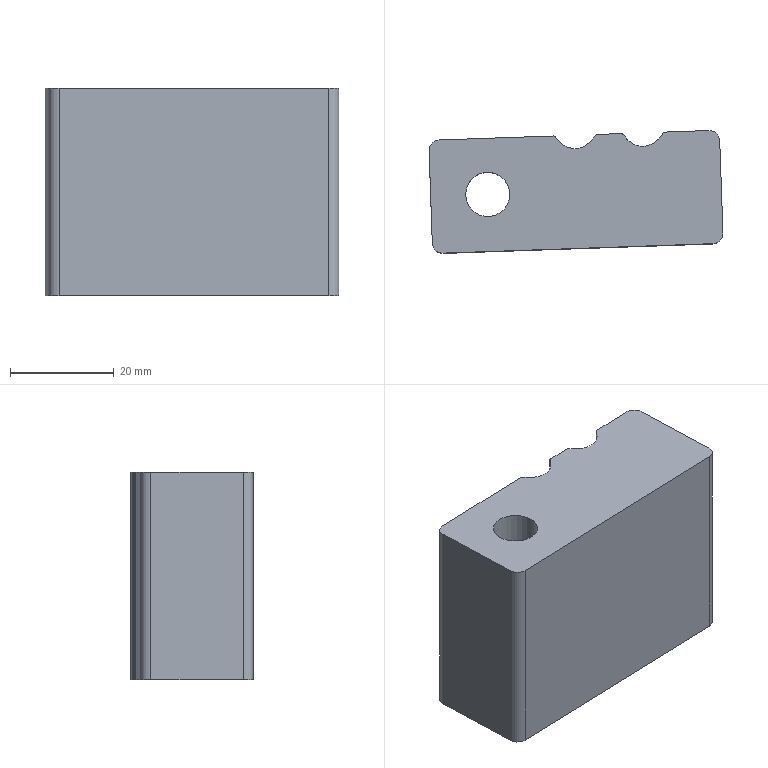Part | NX | features PS-36 2 | 1 solid | 23 faces | box 56.589 x 23.604 x 40 mm | volume 43654 mm3 | cylinder 10 | plane 9 | spline 4 | commonest cylinder face diameters 1 x4 4 x4 8.5 x1 14.5 x1
STEP:
#1=CARTESIAN_POINT('',(3626.085,-818.188,860.716));
#2=VERTEX_POINT('',#1);
#3=CARTESIAN_POINT('',(3648.093,-817.42,860.716));
#4=VERTEX_POINT('',#3);
#5=CARTESIAN_POINT('',(3439.004,-824.721,860.716));
#6=DIRECTION('',(0.9994,0.0349,0.));
#7=VECTOR('',#6,1000.);
#8=LINE('',#5,#7);
#9=EDGE_CURVE('',#2,#4,#8,.T.);
#10=ORIENTED_EDGE('',*,*,#9,.F.);
#11=CARTESIAN_POINT('',(3626.085,-818.188,900.716));
#12=VERTEX_POINT('',#11);
#13=CARTESIAN_POINT('',(3626.085,-818.188,900.716));
#14=DIRECTION('',(0.,0.,1.));
#15=VECTOR('',#14,1000.);
#16=LINE('',#13,#15);
#17=EDGE_CURVE('',#2,#12,#16,.T.);
#18=ORIENTED_EDGE('',*,*,#17,.T.);
#19=CARTESIAN_POINT('',(3648.093,-817.42,900.716));
#20=VERTEX_POINT('',#19);
#21=CARTESIAN_POINT('',(3646.863,-817.463,900.716));
#22=DIRECTION('',(-0.9994,-0.0349,0.));
#23=VECTOR('',#22,1000.);
#24=LINE('',#21,#23);
#25=EDGE_CURVE('',#20,#12,#24,.T.);
#26=ORIENTED_EDGE('',*,*,#25,.F.);
#27=CARTESIAN_POINT('',(3648.093,-817.42,880.716));
#28=DIRECTION('',(0.,0.,1.));
#29=VECTOR('',#28,1000.);
#30=LINE('',#27,#29);
#31=EDGE_CURVE('',#20,#4,#30,.F.);
#32=ORIENTED_EDGE('',*,*,#31,.T.);
#33=EDGE_LOOP('',(#10,#18,#26,#32));
#34=FACE_BOUND('',#33,.T.);
#35=CARTESIAN_POINT('',(3646.863,-817.463,940.716));
#36=DIRECTION('',(0.0349,-0.9994,0.));
#37=DIRECTION('',(-0.9994,-0.0349,0.));
#38=AXIS2_PLACEMENT_3D('',#35,#36,#37);
#39=PLANE('',#38);
#40=ADVANCED_FACE('',(#34),#39,.F.);
#41=CARTESIAN_POINT('',(3648.519,-817.631,900.716));
#42=VERTEX_POINT('',#41);
#43=CARTESIAN_POINT('',(3648.111,-817.92,900.716));
#44=DIRECTION('',(0.,0.,1.));
#45=DIRECTION('',(1.,0.,0.));
#46=AXIS2_PLACEMENT_3D('',#43,#44,#45);
#47=CIRCLE('',#46,0.5);
#48=EDGE_CURVE('',#20,#42,#47,.F.);
#49=ORIENTED_EDGE('',*,*,#48,.T.);
#50=CARTESIAN_POINT('',(3648.519,-817.631,860.716));
#51=VERTEX_POINT('',#50);
#52=CARTESIAN_POINT('',(3648.519,-817.631,860.716));
#53=DIRECTION('',(0.,0.,-1.));
#54=VECTOR('',#53,1000.);
#55=LINE('',#52,#54);
#56=EDGE_CURVE('',#51,#42,#55,.F.);
#57=ORIENTED_EDGE('',*,*,#56,.F.);
#58=CARTESIAN_POINT('',(3648.111,-817.92,860.716));
#59=DIRECTION('',(0.,0.,1.));
#60=DIRECTION('',(1.,0.,0.));
#61=AXIS2_PLACEMENT_3D('',#58,#59,#60);
#62=CIRCLE('',#61,0.5);
#63=EDGE_CURVE('',#4,#51,#62,.F.);
#64=ORIENTED_EDGE('',*,*,#63,.F.);
#65=ORIENTED_EDGE('',*,*,#31,.F.);
#66=EDGE_LOOP('',(#49,#57,#64,#65));
#67=FACE_BOUND('',#66,.T.);
#68=CARTESIAN_POINT('',(3648.111,-817.92,880.716));
#69=DIRECTION('',(0.,0.,-1.));
#70=DIRECTION('',(-1.,0.,0.));
#71=AXIS2_PLACEMENT_3D('',#68,#69,#70);
#72=CYLINDRICAL_SURFACE('',#71,0.5);
#73=ADVANCED_FACE('',(#67),#72,.T.);
#74=CARTESIAN_POINT('',(3652.502,-819.853,900.716));
#75=VERTEX_POINT('',#74);
#76=CARTESIAN_POINT('',(3648.519,-817.631,900.716));
#77=CARTESIAN_POINT('',(3648.979,-818.283,900.716));
#78=CARTESIAN_POINT('',(3650.119,-819.434,900.716));
#79=CARTESIAN_POINT('',(3651.701,-819.895,900.716));
#80=CARTESIAN_POINT('',(3652.502,-819.853,900.716));
#81=B_SPLINE_CURVE_WITH_KNOTS('',3,(#76,#77,#78,#79,#80),.UNSPECIFIED.,.F.,.F.,(4,1,4),(0.,0.002372,0.004744),.UNSPECIFIED.);
#82=EDGE_CURVE('',#42,#75,#81,.T.);
#83=ORIENTED_EDGE('',*,*,#82,.T.);
#84=CARTESIAN_POINT('',(3652.502,-819.853,860.716));
#85=VERTEX_POINT('',#84);
#86=CARTESIAN_POINT('',(3652.502,-819.853,900.716));
#87=CARTESIAN_POINT('',(3652.502,-819.853,887.383));
#88=CARTESIAN_POINT('',(3652.502,-819.853,874.05));
#89=CARTESIAN_POINT('',(3652.502,-819.853,860.716));
#90=B_SPLINE_CURVE_WITH_KNOTS('',3,(#86,#87,#88,#89),.UNSPECIFIED.,.F.,.F.,(4,4),(0.5,1.),.UNSPECIFIED.);
#91=EDGE_CURVE('',#75,#85,#90,.T.);
#92=ORIENTED_EDGE('',*,*,#91,.T.);
#93=CARTESIAN_POINT('',(3652.502,-819.853,860.716));
#94=CARTESIAN_POINT('',(3650.9,-819.937,860.716));
#95=CARTESIAN_POINT('',(3649.439,-818.936,860.716));
#96=CARTESIAN_POINT('',(3648.519,-817.631,860.716));
#97=B_SPLINE_CURVE_WITH_KNOTS('',3,(#93,#94,#95,#96),.UNSPECIFIED.,.F.,.F.,(4,4),(0.,0.004741),.UNSPECIFIED.);
#98=EDGE_CURVE('',#85,#51,#97,.T.);
#99=ORIENTED_EDGE('',*,*,#98,.T.);
#100=ORIENTED_EDGE('',*,*,#56,.T.);
#101=EDGE_LOOP('',(#83,#92,#99,#100));
#102=FACE_BOUND('',#101,.T.);
#103=CARTESIAN_POINT('',(3652.502,-819.853,900.716));
#104=CARTESIAN_POINT('',(3652.502,-819.853,860.716));
#105=CARTESIAN_POINT('',(3652.122,-819.873,900.716));
#106=CARTESIAN_POINT('',(3652.122,-819.873,860.716));
#107=CARTESIAN_POINT('',(3651.27,-819.783,900.716));
#108=CARTESIAN_POINT('',(3651.27,-819.783,860.716));
#109=CARTESIAN_POINT('',(3649.791,-819.109,900.716));
#110=CARTESIAN_POINT('',(3649.791,-819.109,860.716));
#111=CARTESIAN_POINT('',(3648.957,-818.252,900.716));
#112=CARTESIAN_POINT('',(3648.957,-818.252,860.716));
#113=CARTESIAN_POINT('',(3648.519,-817.631,900.716));
#114=CARTESIAN_POINT('',(3648.519,-817.631,860.716));
#115=B_SPLINE_SURFACE_WITH_KNOTS('',3,1,((#103,#104),(#105,#106),(#107,#108),(#109,#110),(#111,#112),(#113,#114)),.SURF_OF_LINEAR_EXTRUSION.,.F.,.F.,.F.,(4,1,1,4),(2,2),(0.,0.2306,0.4611,0.9223),(0.,1.),.UNSPECIFIED.);
#116=ADVANCED_FACE('',(#102),#115,.F.);
#117=CARTESIAN_POINT('',(3656.19,-817.364,900.716));
#118=VERTEX_POINT('',#117);
#119=CARTESIAN_POINT('',(3656.19,-817.364,900.716));
#120=CARTESIAN_POINT('',(3655.385,-818.693,900.716));
#121=CARTESIAN_POINT('',(3654.062,-819.771,900.716));
#122=CARTESIAN_POINT('',(3652.502,-819.853,900.716));
#123=B_SPLINE_CURVE_WITH_KNOTS('',3,(#119,#120,#121,#122),.UNSPECIFIED.,.F.,.F.,(4,4),(0.,0.00462),.UNSPECIFIED.);
#124=EDGE_CURVE('',#118,#75,#123,.T.);
#125=ORIENTED_EDGE('',*,*,#124,.F.);
#126=CARTESIAN_POINT('',(3656.19,-817.364,860.716));
#127=VERTEX_POINT('',#126);
#128=CARTESIAN_POINT('',(3656.19,-817.364,900.716));
#129=DIRECTION('',(0.,0.,-1.));
#130=VECTOR('',#129,1000.);
#131=LINE('',#128,#130);
#132=EDGE_CURVE('',#118,#127,#131,.T.);
#133=ORIENTED_EDGE('',*,*,#132,.T.);
#134=CARTESIAN_POINT('',(3656.19,-817.364,860.716));
#135=CARTESIAN_POINT('',(3655.385,-818.693,860.716));
#136=CARTESIAN_POINT('',(3654.062,-819.771,860.716));
#137=CARTESIAN_POINT('',(3652.502,-819.853,860.716));
#138=B_SPLINE_CURVE_WITH_KNOTS('',3,(#134,#135,#136,#137),.UNSPECIFIED.,.F.,.F.,(4,4),(0.,0.00462),.UNSPECIFIED.);
#139=EDGE_CURVE('',#127,#85,#138,.T.);
#140=ORIENTED_EDGE('',*,*,#139,.T.);
#141=ORIENTED_EDGE('',*,*,#91,.F.);
#142=EDGE_LOOP('',(#125,#133,#140,#141));
#143=FACE_BOUND('',#142,.T.);
#144=CARTESIAN_POINT('',(3656.19,-817.364,900.716));
#145=CARTESIAN_POINT('',(3656.19,-817.364,860.716));
#146=CARTESIAN_POINT('',(3655.806,-817.996,900.716));
#147=CARTESIAN_POINT('',(3655.806,-817.996,860.716));
#148=CARTESIAN_POINT('',(3654.845,-819.188,900.716));
#149=CARTESIAN_POINT('',(3654.845,-819.188,860.716));
#150=CARTESIAN_POINT('',(3653.241,-819.814,900.716));
#151=CARTESIAN_POINT('',(3653.241,-819.814,860.716));
#152=CARTESIAN_POINT('',(3652.502,-819.853,900.716));
#153=CARTESIAN_POINT('',(3652.502,-819.853,860.716));
#154=B_SPLINE_SURFACE_WITH_KNOTS('',3,1,((#144,#145),(#146,#147),(#148,#149),(#150,#151),(#152,#153)),.SURF_OF_LINEAR_EXTRUSION.,.F.,.F.,.F.,(4,1,4),(2,2),(0.07964,0.5398,1.),(0.,1.),.UNSPECIFIED.);
#155=ADVANCED_FACE('',(#143),#154,.F.);
#156=CARTESIAN_POINT('',(3656.6,-817.123,900.716));
#157=VERTEX_POINT('',#156);
#158=CARTESIAN_POINT('',(3656.617,-817.623,900.716));
#159=DIRECTION('',(0.,0.,1.));
#160=DIRECTION('',(1.,0.,0.));
#161=AXIS2_PLACEMENT_3D('',#158,#159,#160);
#162=CIRCLE('',#161,0.5);
#163=EDGE_CURVE('',#157,#118,#162,.T.);
#164=ORIENTED_EDGE('',*,*,#163,.F.);
#165=CARTESIAN_POINT('',(3656.6,-817.123,860.716));
#166=VERTEX_POINT('',#165);
#167=CARTESIAN_POINT('',(3656.6,-817.123,880.716));
#168=DIRECTION('',(0.,0.,1.));
#169=VECTOR('',#168,1000.);
#170=LINE('',#167,#169);
#171=EDGE_CURVE('',#166,#157,#170,.T.);
#172=ORIENTED_EDGE('',*,*,#171,.F.);
#173=CARTESIAN_POINT('',(3656.617,-817.623,860.716));
#174=DIRECTION('',(0.,0.,1.));
#175=DIRECTION('',(1.,0.,0.));
#176=AXIS2_PLACEMENT_3D('',#173,#174,#175);
#177=CIRCLE('',#176,0.5);
#178=EDGE_CURVE('',#127,#166,#177,.F.);
#179=ORIENTED_EDGE('',*,*,#178,.F.);
#180=ORIENTED_EDGE('',*,*,#132,.F.);
#181=EDGE_LOOP('',(#164,#172,#179,#180));
#182=FACE_BOUND('',#181,.T.);
#183=CARTESIAN_POINT('',(3656.617,-817.623,880.716));
#184=DIRECTION('',(0.,0.,-1.));
#185=DIRECTION('',(-1.,0.,0.));
#186=AXIS2_PLACEMENT_3D('',#183,#184,#185);
#187=CYLINDRICAL_SURFACE('',#186,0.5);
#188=ADVANCED_FACE('',(#182),#187,.T.);
#189=CARTESIAN_POINT('',(3661.085,-816.966,900.716));
#190=VERTEX_POINT('',#189);
#191=CARTESIAN_POINT('',(3661.085,-816.966,860.716));
#192=VERTEX_POINT('',#191);
#193=CARTESIAN_POINT('',(3661.085,-816.966,880.716));
#194=DIRECTION('',(0.,0.,1.));
#195=VECTOR('',#194,1000.);
#196=LINE('',#193,#195);
#197=EDGE_CURVE('',#190,#192,#196,.F.);
#198=ORIENTED_EDGE('',*,*,#197,.T.);
#199=CARTESIAN_POINT('',(3439.004,-824.721,860.716));
#200=DIRECTION('',(0.9994,0.0349,0.));
#201=VECTOR('',#200,1000.);
#202=LINE('',#199,#201);
#203=EDGE_CURVE('',#166,#192,#202,.T.);
#204=ORIENTED_EDGE('',*,*,#203,.F.);
#205=ORIENTED_EDGE('',*,*,#171,.T.);
#206=CARTESIAN_POINT('',(3658.843,-817.045,900.716));
#207=DIRECTION('',(0.9994,0.0349,0.));
#208=VECTOR('',#207,1000.);
#209=LINE('',#206,#208);
#210=EDGE_CURVE('',#157,#190,#209,.T.);
#211=ORIENTED_EDGE('',*,*,#210,.T.);
#212=EDGE_LOOP('',(#198,#204,#205,#211));
#213=FACE_BOUND('',#212,.T.);
#214=CARTESIAN_POINT('',(3658.843,-817.045,940.716));
#215=DIRECTION('',(0.0349,-0.9994,0.));
#216=DIRECTION('',(-0.9994,-0.0349,0.));
#217=AXIS2_PLACEMENT_3D('',#214,#215,#216);
#218=PLANE('',#217);
#219=ADVANCED_FACE('',(#213),#218,.F.);
#220=CARTESIAN_POINT('',(3661.511,-817.178,900.716));
#221=VERTEX_POINT('',#220);
#222=CARTESIAN_POINT('',(3661.103,-817.466,900.716));
#223=DIRECTION('',(0.,0.,1.));
#224=DIRECTION('',(1.,0.,0.));
#225=AXIS2_PLACEMENT_3D('',#222,#223,#224);
#226=CIRCLE('',#225,0.5);
#227=EDGE_CURVE('',#221,#190,#226,.T.);
#228=ORIENTED_EDGE('',*,*,#227,.F.);
#229=CARTESIAN_POINT('',(3661.511,-817.178,860.716));
#230=VERTEX_POINT('',#229);
#231=CARTESIAN_POINT('',(3661.511,-817.178,860.716));
#232=DIRECTION('',(0.,0.,-1.));
#233=VECTOR('',#232,1000.);
#234=LINE('',#231,#233);
#235=EDGE_CURVE('',#230,#221,#234,.F.);
#236=ORIENTED_EDGE('',*,*,#235,.F.);
#237=CARTESIAN_POINT('',(3661.103,-817.466,860.716));
#238=DIRECTION('',(0.,0.,1.));
#239=DIRECTION('',(1.,0.,0.));
#240=AXIS2_PLACEMENT_3D('',#237,#238,#239);
#241=CIRCLE('',#240,0.5);
#242=EDGE_CURVE('',#192,#230,#241,.F.);
#243=ORIENTED_EDGE('',*,*,#242,.F.);
#244=ORIENTED_EDGE('',*,*,#197,.F.);
#245=EDGE_LOOP('',(#228,#236,#243,#244));
#246=FACE_BOUND('',#245,.T.);
#247=CARTESIAN_POINT('',(3661.103,-817.466,880.716));
#248=DIRECTION('',(0.,0.,-1.));
#249=DIRECTION('',(-1.,0.,0.));
#250=AXIS2_PLACEMENT_3D('',#247,#248,#249);
#251=CYLINDRICAL_SURFACE('',#250,0.5);
#252=ADVANCED_FACE('',(#246),#251,.T.);
#253=CARTESIAN_POINT('',(3665.494,-819.399,900.716));
#254=VERTEX_POINT('',#253);
#255=CARTESIAN_POINT('',(3661.511,-817.178,900.716));
#256=CARTESIAN_POINT('',(3661.971,-817.83,900.716));
#257=CARTESIAN_POINT('',(3663.111,-818.98,900.716));
#258=CARTESIAN_POINT('',(3664.693,-819.441,900.716));
#259=CARTESIAN_POINT('',(3665.494,-819.399,900.716));
#260=B_SPLINE_CURVE_WITH_KNOTS('',3,(#255,#256,#257,#258,#259),.UNSPECIFIED.,.F.,.F.,(4,1,4),(0.,0.002372,0.004744),.UNSPECIFIED.);
#261=EDGE_CURVE('',#221,#254,#260,.T.);
#262=ORIENTED_EDGE('',*,*,#261,.T.);
#263=CARTESIAN_POINT('',(3665.494,-819.399,860.716));
#264=VERTEX_POINT('',#263);
#265=CARTESIAN_POINT('',(3665.494,-819.399,900.716));
#266=CARTESIAN_POINT('',(3665.494,-819.399,887.383));
#267=CARTESIAN_POINT('',(3665.494,-819.399,874.05));
#268=CARTESIAN_POINT('',(3665.494,-819.399,860.716));
#269=B_SPLINE_CURVE_WITH_KNOTS('',3,(#265,#266,#267,#268),.UNSPECIFIED.,.F.,.F.,(4,4),(0.5,1.),.UNSPECIFIED.);
#270=EDGE_CURVE('',#254,#264,#269,.T.);
#271=ORIENTED_EDGE('',*,*,#270,.T.);
#272=CARTESIAN_POINT('',(3665.494,-819.399,860.716));
#273=CARTESIAN_POINT('',(3663.892,-819.483,860.716));
#274=CARTESIAN_POINT('',(3662.431,-818.482,860.716));
#275=CARTESIAN_POINT('',(3661.511,-817.178,860.716));
#276=B_SPLINE_CURVE_WITH_KNOTS('',3,(#272,#273,#274,#275),.UNSPECIFIED.,.F.,.F.,(4,4),(0.,0.004741),.UNSPECIFIED.);
#277=EDGE_CURVE('',#264,#230,#276,.T.);
#278=ORIENTED_EDGE('',*,*,#277,.T.);
#279=ORIENTED_EDGE('',*,*,#235,.T.);
#280=EDGE_LOOP('',(#262,#271,#278,#279));
#281=FACE_BOUND('',#280,.T.);
#282=CARTESIAN_POINT('',(3665.494,-819.399,900.716));
#283=CARTESIAN_POINT('',(3665.494,-819.399,860.716));
#284=CARTESIAN_POINT('',(3665.115,-819.419,900.716));
#285=CARTESIAN_POINT('',(3665.115,-819.419,860.716));
#286=CARTESIAN_POINT('',(3664.262,-819.33,900.716));
#287=CARTESIAN_POINT('',(3664.262,-819.33,860.716));
#288=CARTESIAN_POINT('',(3662.783,-818.655,900.716));
#289=CARTESIAN_POINT('',(3662.783,-818.655,860.716));
#290=CARTESIAN_POINT('',(3661.949,-817.799,900.716));
#291=CARTESIAN_POINT('',(3661.949,-817.799,860.716));
#292=CARTESIAN_POINT('',(3661.511,-817.178,900.716));
#293=CARTESIAN_POINT('',(3661.511,-817.178,860.716));
#294=B_SPLINE_SURFACE_WITH_KNOTS('',3,1,((#282,#283),(#284,#285),(#286,#287),(#288,#289),(#290,#291),(#292,#293)),.SURF_OF_LINEAR_EXTRUSION.,.F.,.F.,.F.,(4,1,1,4),(2,2),(-0.000000001,0.2306,0.4611,0.9223),(0.,1.),.UNSPECIFIED.);
#295=ADVANCED_FACE('',(#281),#294,.F.);
#296=CARTESIAN_POINT('',(3669.182,-816.91,900.716));
#297=VERTEX_POINT('',#296);
#298=CARTESIAN_POINT('',(3669.182,-816.91,900.716));
#299=CARTESIAN_POINT('',(3668.377,-818.239,900.716));
#300=CARTESIAN_POINT('',(3667.054,-819.317,900.716));
#301=CARTESIAN_POINT('',(3665.494,-819.399,900.716));
#302=B_SPLINE_CURVE_WITH_KNOTS('',3,(#298,#299,#300,#301),.UNSPECIFIED.,.F.,.F.,(4,4),(0.,0.00462),.UNSPECIFIED.);
#303=EDGE_CURVE('',#297,#254,#302,.T.);
#304=ORIENTED_EDGE('',*,*,#303,.F.);
#305=CARTESIAN_POINT('',(3669.182,-816.91,860.716));
#306=VERTEX_POINT('',#305);
#307=CARTESIAN_POINT('',(3669.182,-816.91,900.716));
#308=DIRECTION('',(0.,0.,-1.));
#309=VECTOR('',#308,1000.);
#310=LINE('',#307,#309);
#311=EDGE_CURVE('',#297,#306,#310,.T.);
#312=ORIENTED_EDGE('',*,*,#311,.T.);
#313=CARTESIAN_POINT('',(3669.182,-816.91,860.716));
#314=CARTESIAN_POINT('',(3668.377,-818.239,860.716));
#315=CARTESIAN_POINT('',(3667.054,-819.317,860.716));
#316=CARTESIAN_POINT('',(3665.494,-819.399,860.716));
#317=B_SPLINE_CURVE_WITH_KNOTS('',3,(#313,#314,#315,#316),.UNSPECIFIED.,.F.,.F.,(4,4),(0.,0.00462),.UNSPECIFIED.);
#318=EDGE_CURVE('',#306,#264,#317,.T.);
#319=ORIENTED_EDGE('',*,*,#318,.T.);
#320=ORIENTED_EDGE('',*,*,#270,.F.);
#321=EDGE_LOOP('',(#304,#312,#319,#320));
#322=FACE_BOUND('',#321,.T.);
#323=CARTESIAN_POINT('',(3669.195,-816.887,900.716));
#324=CARTESIAN_POINT('',(3669.195,-816.887,860.716));
#325=CARTESIAN_POINT('',(3668.813,-817.525,900.716));
#326=CARTESIAN_POINT('',(3668.813,-817.525,860.716));
#327=CARTESIAN_POINT('',(3668.064,-818.423,900.716));
#328=CARTESIAN_POINT('',(3668.064,-818.423,860.716));
#329=CARTESIAN_POINT('',(3666.686,-819.208,900.716));
#330=CARTESIAN_POINT('',(3666.686,-819.208,860.716));
#331=CARTESIAN_POINT('',(3665.866,-819.38,900.716));
#332=CARTESIAN_POINT('',(3665.866,-819.38,860.716));
#333=CARTESIAN_POINT('',(3665.494,-819.399,900.716));
#334=CARTESIAN_POINT('',(3665.494,-819.399,860.716));
#335=B_SPLINE_SURFACE_WITH_KNOTS('',3,1,((#323,#324),(#325,#326),(#327,#328),(#329,#330),(#331,#332),(#333,#334)),.SURF_OF_LINEAR_EXTRUSION.,.F.,.F.,.F.,(4,1,1,4),(2,2),(0.07412,0.5371,0.7685,1.),(0.,1.),.UNSPECIFIED.);
#336=ADVANCED_FACE('',(#322),#335,.F.);
#337=CARTESIAN_POINT('',(3669.592,-816.669,900.716));
#338=VERTEX_POINT('',#337);
#339=CARTESIAN_POINT('',(3669.609,-817.169,900.716));
#340=DIRECTION('',(0.,0.,1.));
#341=DIRECTION('',(1.,0.,0.));
#342=AXIS2_PLACEMENT_3D('',#339,#340,#341);
#343=CIRCLE('',#342,0.5);
#344=EDGE_CURVE('',#297,#338,#343,.F.);
#345=ORIENTED_EDGE('',*,*,#344,.T.);
#346=CARTESIAN_POINT('',(3669.592,-816.669,860.716));
#347=VERTEX_POINT('',#346);
#348=CARTESIAN_POINT('',(3669.592,-816.669,880.716));
#349=DIRECTION('',(0.,0.,1.));
#350=VECTOR('',#349,1000.);
#351=LINE('',#348,#350);
#352=EDGE_CURVE('',#347,#338,#351,.T.);
#353=ORIENTED_EDGE('',*,*,#352,.F.);
#354=CARTESIAN_POINT('',(3669.609,-817.169,860.716));
#355=DIRECTION('',(0.,0.,1.));
#356=DIRECTION('',(1.,0.,0.));
#357=AXIS2_PLACEMENT_3D('',#354,#355,#356);
#358=CIRCLE('',#357,0.5);
#359=EDGE_CURVE('',#306,#347,#358,.F.);
#360=ORIENTED_EDGE('',*,*,#359,.F.);
#361=ORIENTED_EDGE('',*,*,#311,.F.);
#362=EDGE_LOOP('',(#345,#353,#360,#361));
#363=FACE_BOUND('',#362,.T.);
#364=CARTESIAN_POINT('',(3669.609,-817.169,880.716));
#365=DIRECTION('',(0.,0.,-1.));
#366=DIRECTION('',(-1.,0.,0.));
#367=AXIS2_PLACEMENT_3D('',#364,#365,#366);
#368=CYLINDRICAL_SURFACE('',#367,0.5);
#369=ADVANCED_FACE('',(#363),#368,.T.);
#370=CARTESIAN_POINT('',(3678.053,-816.374,900.716));
#371=VERTEX_POINT('',#370);
#372=CARTESIAN_POINT('',(3658.843,-817.045,900.716));
#373=DIRECTION('',(0.9994,0.0349,0.));
#374=VECTOR('',#373,1000.);
#375=LINE('',#372,#374);
#376=EDGE_CURVE('',#338,#371,#375,.T.);
#377=ORIENTED_EDGE('',*,*,#376,.T.);
#378=CARTESIAN_POINT('',(3678.053,-816.374,860.716));
#379=VERTEX_POINT('',#378);
#380=CARTESIAN_POINT('',(3678.053,-816.374,860.716));
#381=DIRECTION('',(0.,0.,-1.));
#382=VECTOR('',#381,1000.);
#383=LINE('',#380,#382);
#384=EDGE_CURVE('',#371,#379,#383,.T.);
#385=ORIENTED_EDGE('',*,*,#384,.T.);
#386=CARTESIAN_POINT('',(3439.004,-824.721,860.716));
#387=DIRECTION('',(0.9994,0.0349,0.));
#388=VECTOR('',#387,1000.);
#389=LINE('',#386,#388);
#390=EDGE_CURVE('',#347,#379,#389,.T.);
#391=ORIENTED_EDGE('',*,*,#390,.F.);
#392=ORIENTED_EDGE('',*,*,#352,.T.);
#393=EDGE_LOOP('',(#377,#385,#391,#392));
#394=FACE_BOUND('',#393,.T.);
#395=CARTESIAN_POINT('',(3661.467,-816.953,940.716));
#396=DIRECTION('',(0.0349,-0.9994,0.));
#397=DIRECTION('',(-0.9994,-0.0349,0.));
#398=AXIS2_PLACEMENT_3D('',#395,#396,#397);
#399=PLANE('',#398);
#400=ADVANCED_FACE('',(#394),#399,.F.);
#401=CARTESIAN_POINT('',(3680.743,-836.092,900.716));
#402=VERTEX_POINT('',#401);
#403=CARTESIAN_POINT('',(3680.122,-818.303,900.716));
#404=VERTEX_POINT('',#403);
#405=CARTESIAN_POINT('',(3680.917,-841.089,900.716));
#406=DIRECTION('',(-0.0349,0.9994,0.));
#407=VECTOR('',#406,1000.);
#408=LINE('',#405,#407);
#409=EDGE_CURVE('',#402,#404,#408,.T.);
#410=ORIENTED_EDGE('',*,*,#409,.F.);
#411=CARTESIAN_POINT('',(3680.743,-836.092,860.716));
#412=VERTEX_POINT('',#411);
#413=CARTESIAN_POINT('',(3680.743,-836.092,860.716));
#414=DIRECTION('',(0.,0.,-1.));
#415=VECTOR('',#414,1000.);
#416=LINE('',#413,#415);
#417=EDGE_CURVE('',#402,#412,#416,.T.);
#418=ORIENTED_EDGE('',*,*,#417,.T.);
#419=CARTESIAN_POINT('',(3680.122,-818.303,860.716));
#420=VERTEX_POINT('',#419);
#421=CARTESIAN_POINT('',(3686.141,-990.705,860.716));
#422=DIRECTION('',(-0.0349,0.9994,0.));
#423=VECTOR('',#422,1000.);
#424=LINE('',#421,#423);
#425=EDGE_CURVE('',#412,#420,#424,.T.);
#426=ORIENTED_EDGE('',*,*,#425,.T.);
#427=CARTESIAN_POINT('',(3680.122,-818.303,900.716));
#428=DIRECTION('',(0.,0.,-1.));
#429=VECTOR('',#428,1000.);
#430=LINE('',#427,#429);
#431=EDGE_CURVE('',#420,#404,#430,.F.);
#432=ORIENTED_EDGE('',*,*,#431,.T.);
#433=EDGE_LOOP('',(#410,#418,#426,#432));
#434=FACE_BOUND('',#433,.T.);
#435=CARTESIAN_POINT('',(3680.917,-841.089,940.716));
#436=DIRECTION('',(0.9994,0.0349,0.));
#437=DIRECTION('',(-0.0349,0.9994,0.));
#438=AXIS2_PLACEMENT_3D('',#435,#436,#437);
#439=PLANE('',#438);
#440=ADVANCED_FACE('',(#434),#439,.T.);
#441=CARTESIAN_POINT('',(3642.706,-828.668,860.716));
#442=VERTEX_POINT('',#441);
#443=CARTESIAN_POINT('',(3635.456,-828.668,860.716));
#444=DIRECTION('',(0.,0.,1.));
#445=DIRECTION('',(1.,0.,0.));
#446=AXIS2_PLACEMENT_3D('',#443,#444,#445);
#447=CIRCLE('',#446,7.25);
#448=EDGE_CURVE('',#442,#442,#447,.T.);
#449=ORIENTED_EDGE('',*,*,#448,.T.);
#450=EDGE_LOOP('',(#449));
#451=FACE_BOUND('',#450,.T.);
#452=ORIENTED_EDGE('',*,*,#425,.F.);
#453=CARTESIAN_POINT('',(3678.814,-838.161,860.716));
#454=VERTEX_POINT('',#453);
#455=CARTESIAN_POINT('',(3678.744,-836.162,860.716));
#456=DIRECTION('',(0.,0.,1.));
#457=DIRECTION('',(1.,0.,0.));
#458=AXIS2_PLACEMENT_3D('',#455,#456,#457);
#459=CIRCLE('',#458,2.);
#460=EDGE_CURVE('',#412,#454,#459,.F.);
#461=ORIENTED_EDGE('',*,*,#460,.T.);
#462=CARTESIAN_POINT('',(3626.845,-839.975,860.716));
#463=VERTEX_POINT('',#462);
#464=CARTESIAN_POINT('',(3439.765,-846.507,860.716));
#465=DIRECTION('',(-0.9994,-0.0349,0.));
#466=VECTOR('',#465,1000.);
#467=LINE('',#464,#466);
#468=EDGE_CURVE('',#454,#463,#467,.T.);
#469=ORIENTED_EDGE('',*,*,#468,.T.);
#470=CARTESIAN_POINT('',(3624.777,-838.046,860.716));
#471=VERTEX_POINT('',#470);
#472=CARTESIAN_POINT('',(3626.776,-837.976,860.716));
#473=DIRECTION('',(0.,0.,1.));
#474=DIRECTION('',(1.,0.,0.));
#475=AXIS2_PLACEMENT_3D('',#472,#473,#474);
#476=CIRCLE('',#475,2.);
#477=EDGE_CURVE('',#463,#471,#476,.F.);
#478=ORIENTED_EDGE('',*,*,#477,.T.);
#479=CARTESIAN_POINT('',(3624.156,-820.257,860.716));
#480=VERTEX_POINT('',#479);
#481=CARTESIAN_POINT('',(3624.951,-843.043,860.716));
#482=DIRECTION('',(-0.0349,0.9994,0.));
#483=VECTOR('',#482,1000.);
#484=LINE('',#481,#483);
#485=EDGE_CURVE('',#471,#480,#484,.T.);
#486=ORIENTED_EDGE('',*,*,#485,.T.);
#487=CARTESIAN_POINT('',(3626.154,-820.187,860.716));
#488=DIRECTION('',(0.,0.,1.));
#489=DIRECTION('',(1.,0.,0.));
#490=AXIS2_PLACEMENT_3D('',#487,#488,#489);
#491=CIRCLE('',#490,2.);
#492=EDGE_CURVE('',#480,#2,#491,.F.);
#493=ORIENTED_EDGE('',*,*,#492,.T.);
#494=ORIENTED_EDGE('',*,*,#9,.T.);
#495=ORIENTED_EDGE('',*,*,#63,.T.);
#496=ORIENTED_EDGE('',*,*,#98,.F.);
#497=ORIENTED_EDGE('',*,*,#139,.F.);
#498=ORIENTED_EDGE('',*,*,#178,.T.);
#499=ORIENTED_EDGE('',*,*,#203,.T.);
#500=ORIENTED_EDGE('',*,*,#242,.T.);
#501=ORIENTED_EDGE('',*,*,#277,.F.);
#502=ORIENTED_EDGE('',*,*,#318,.F.);
#503=ORIENTED_EDGE('',*,*,#359,.T.);
#504=ORIENTED_EDGE('',*,*,#390,.T.);
#505=CARTESIAN_POINT('',(3678.123,-818.373,860.716));
#506=DIRECTION('',(0.,0.,1.));
#507=DIRECTION('',(1.,0.,0.));
#508=AXIS2_PLACEMENT_3D('',#505,#506,#507);
#509=CIRCLE('',#508,2.);
#510=EDGE_CURVE('',#379,#420,#509,.F.);
#511=ORIENTED_EDGE('',*,*,#510,.T.);
#512=EDGE_LOOP('',(#452,#461,#469,#478,#486,#493,#494,#495,#496,#497,#498,#499,#500,#501,#502,#503,#504,#511));
#513=FACE_BOUND('',#512,.T.);
#514=CARTESIAN_POINT('',(3445.094,-999.122,860.716));
#515=DIRECTION('',(0.,0.,1.));
#516=DIRECTION('',(0.,1.,0.));
#517=AXIS2_PLACEMENT_3D('',#514,#515,#516);
#518=PLANE('',#517);
#519=ADVANCED_FACE('',(#451,#513),#518,.F.);
#520=ORIENTED_EDGE('',*,*,#485,.F.);
#521=CARTESIAN_POINT('',(3624.777,-838.046,900.716));
#522=VERTEX_POINT('',#521);
#523=CARTESIAN_POINT('',(3624.777,-838.046,900.716));
#524=DIRECTION('',(0.,0.,1.));
#525=VECTOR('',#524,1000.);
#526=LINE('',#523,#525);
#527=EDGE_CURVE('',#471,#522,#526,.T.);
#528=ORIENTED_EDGE('',*,*,#527,.T.);
#529=CARTESIAN_POINT('',(3624.156,-820.257,900.716));
#530=VERTEX_POINT('',#529);
#531=CARTESIAN_POINT('',(3624.951,-843.043,900.716));
#532=DIRECTION('',(-0.0349,0.9994,0.));
#533=VECTOR('',#532,1000.);
#534=LINE('',#531,#533);
#535=EDGE_CURVE('',#522,#530,#534,.T.);
#536=ORIENTED_EDGE('',*,*,#535,.T.);
#537=CARTESIAN_POINT('',(3624.156,-820.257,860.716));
#538=DIRECTION('',(0.,0.,1.));
#539=VECTOR('',#538,1000.);
#540=LINE('',#537,#539);
#541=EDGE_CURVE('',#530,#480,#540,.F.);
#542=ORIENTED_EDGE('',*,*,#541,.T.);
#543=EDGE_LOOP('',(#520,#528,#536,#542));
#544=FACE_BOUND('',#543,.T.);
#545=CARTESIAN_POINT('',(3624.951,-843.043,940.716));
#546=DIRECTION('',(-0.9994,-0.0349,0.));
#547=DIRECTION('',(0.0349,-0.9994,0.));
#548=AXIS2_PLACEMENT_3D('',#545,#546,#547);
#549=PLANE('',#548);
#550=ADVANCED_FACE('',(#544),#549,.T.);
#551=CARTESIAN_POINT('',(3639.706,-828.668,900.716));
#552=VERTEX_POINT('',#551);
#553=CARTESIAN_POINT('',(3635.456,-828.668,900.716));
#554=DIRECTION('',(0.,0.,1.));
#555=DIRECTION('',(1.,0.,0.));
#556=AXIS2_PLACEMENT_3D('',#553,#554,#555);
#557=CIRCLE('',#556,4.25);
#558=EDGE_CURVE('',#552,#552,#557,.T.);
#559=ORIENTED_EDGE('',*,*,#558,.F.);
#560=EDGE_LOOP('',(#559));
#561=FACE_BOUND('',#560,.T.);
#562=ORIENTED_EDGE('',*,*,#535,.F.);
#563=CARTESIAN_POINT('',(3626.845,-839.975,900.716));
#564=VERTEX_POINT('',#563);
#565=CARTESIAN_POINT('',(3626.776,-837.976,900.716));
#566=DIRECTION('',(0.,0.,1.));
#567=DIRECTION('',(1.,0.,0.));
#568=AXIS2_PLACEMENT_3D('',#565,#566,#567);
#569=CIRCLE('',#568,2.);
#570=EDGE_CURVE('',#522,#564,#569,.T.);
#571=ORIENTED_EDGE('',*,*,#570,.T.);
#572=CARTESIAN_POINT('',(3678.814,-838.161,900.716));
#573=VERTEX_POINT('',#572);
#574=CARTESIAN_POINT('',(3659.603,-838.831,900.716));
#575=DIRECTION('',(-0.9994,-0.0349,0.));
#576=VECTOR('',#575,1000.);
#577=LINE('',#574,#576);
#578=EDGE_CURVE('',#573,#564,#577,.T.);
#579=ORIENTED_EDGE('',*,*,#578,.F.);
#580=CARTESIAN_POINT('',(3678.744,-836.162,900.716));
#581=DIRECTION('',(0.,0.,1.));
#582=DIRECTION('',(1.,0.,0.));
#583=AXIS2_PLACEMENT_3D('',#580,#581,#582);
#584=CIRCLE('',#583,2.);
#585=EDGE_CURVE('',#573,#402,#584,.T.);
#586=ORIENTED_EDGE('',*,*,#585,.T.);
#587=ORIENTED_EDGE('',*,*,#409,.T.);
#588=CARTESIAN_POINT('',(3678.123,-818.373,900.716));
#589=DIRECTION('',(0.,0.,1.));
#590=DIRECTION('',(1.,0.,0.));
#591=AXIS2_PLACEMENT_3D('',#588,#589,#590);
#592=CIRCLE('',#591,2.);
#593=EDGE_CURVE('',#404,#371,#592,.T.);
#594=ORIENTED_EDGE('',*,*,#593,.T.);
#595=ORIENTED_EDGE('',*,*,#376,.F.);
#596=ORIENTED_EDGE('',*,*,#344,.F.);
#597=ORIENTED_EDGE('',*,*,#303,.T.);
#598=ORIENTED_EDGE('',*,*,#261,.F.);
#599=ORIENTED_EDGE('',*,*,#227,.T.);
#600=ORIENTED_EDGE('',*,*,#210,.F.);
#601=ORIENTED_EDGE('',*,*,#163,.T.);
#602=ORIENTED_EDGE('',*,*,#124,.T.);
#603=ORIENTED_EDGE('',*,*,#82,.F.);
#604=ORIENTED_EDGE('',*,*,#48,.F.);
#605=ORIENTED_EDGE('',*,*,#25,.T.);
#606=CARTESIAN_POINT('',(3626.154,-820.187,900.716));
#607=DIRECTION('',(0.,0.,1.));
#608=DIRECTION('',(1.,0.,0.));
#609=AXIS2_PLACEMENT_3D('',#606,#607,#608);
#610=CIRCLE('',#609,2.);
#611=EDGE_CURVE('',#12,#530,#610,.T.);
#612=ORIENTED_EDGE('',*,*,#611,.T.);
#613=EDGE_LOOP('',(#562,#571,#579,#586,#587,#594,#595,#596,#597,#598,#599,#600,#601,#602,#603,#604,#605,#612));
#614=FACE_BOUND('',#613,.T.);
#615=CARTESIAN_POINT('',(3659.708,-841.829,900.716));
#616=DIRECTION('',(0.,0.,1.));
#617=DIRECTION('',(1.,0.,0.));
#618=AXIS2_PLACEMENT_3D('',#615,#616,#617);
#619=PLANE('',#618);
#620=ADVANCED_FACE('',(#561,#614),#619,.T.);
#621=ORIENTED_EDGE('',*,*,#578,.T.);
#622=CARTESIAN_POINT('',(3626.845,-839.975,860.716));
#623=DIRECTION('',(0.,0.,1.));
#624=VECTOR('',#623,1000.);
#625=LINE('',#622,#624);
#626=EDGE_CURVE('',#564,#463,#625,.F.);
#627=ORIENTED_EDGE('',*,*,#626,.T.);
#628=ORIENTED_EDGE('',*,*,#468,.F.);
#629=CARTESIAN_POINT('',(3678.814,-838.161,900.716));
#630=DIRECTION('',(0.,0.,-1.));
#631=VECTOR('',#630,1000.);
#632=LINE('',#629,#631);
#633=EDGE_CURVE('',#454,#573,#632,.F.);
#634=ORIENTED_EDGE('',*,*,#633,.T.);
#635=EDGE_LOOP('',(#621,#627,#628,#634));
#636=FACE_BOUND('',#635,.T.);
#637=CARTESIAN_POINT('',(3675.528,-838.275,880.715));
#638=DIRECTION('',(-0.0349,0.9994,0.));
#639=DIRECTION('',(-0.9994,-0.0349,0.));
#640=AXIS2_PLACEMENT_3D('',#637,#638,#639);
#641=PLANE('',#640);
#642=ADVANCED_FACE('',(#636),#641,.F.);
#643=ORIENTED_EDGE('',*,*,#477,.F.);
#644=ORIENTED_EDGE('',*,*,#626,.F.);
#645=ORIENTED_EDGE('',*,*,#570,.F.);
#646=ORIENTED_EDGE('',*,*,#527,.F.);
#647=EDGE_LOOP('',(#643,#644,#645,#646));
#648=FACE_BOUND('',#647,.T.);
#649=CARTESIAN_POINT('',(3626.776,-837.976,940.716));
#650=DIRECTION('',(0.,0.,-1.));
#651=DIRECTION('',(-1.,0.,0.));
#652=AXIS2_PLACEMENT_3D('',#649,#650,#651);
#653=CYLINDRICAL_SURFACE('',#652,2.);
#654=ADVANCED_FACE('',(#648),#653,.T.);
#655=ORIENTED_EDGE('',*,*,#492,.F.);
#656=ORIENTED_EDGE('',*,*,#541,.F.);
#657=ORIENTED_EDGE('',*,*,#611,.F.);
#658=ORIENTED_EDGE('',*,*,#17,.F.);
#659=EDGE_LOOP('',(#655,#656,#657,#658));
#660=FACE_BOUND('',#659,.T.);
#661=CARTESIAN_POINT('',(3626.154,-820.187,940.716));
#662=DIRECTION('',(0.,0.,-1.));
#663=DIRECTION('',(-1.,0.,0.));
#664=AXIS2_PLACEMENT_3D('',#661,#662,#663);
#665=CYLINDRICAL_SURFACE('',#664,2.);
#666=ADVANCED_FACE('',(#660),#665,.T.);
#667=ORIENTED_EDGE('',*,*,#585,.F.);
#668=ORIENTED_EDGE('',*,*,#633,.F.);
#669=ORIENTED_EDGE('',*,*,#460,.F.);
#670=ORIENTED_EDGE('',*,*,#417,.F.);
#671=EDGE_LOOP('',(#667,#668,#669,#670));
#672=FACE_BOUND('',#671,.T.);
#673=CARTESIAN_POINT('',(3678.744,-836.162,940.716));
#674=DIRECTION('',(0.,0.,1.));
#675=DIRECTION('',(1.,0.,0.));
#676=AXIS2_PLACEMENT_3D('',#673,#674,#675);
#677=CYLINDRICAL_SURFACE('',#676,2.);
#678=ADVANCED_FACE('',(#672),#677,.T.);
#679=ORIENTED_EDGE('',*,*,#593,.F.);
#680=ORIENTED_EDGE('',*,*,#431,.F.);
#681=ORIENTED_EDGE('',*,*,#510,.F.);
#682=ORIENTED_EDGE('',*,*,#384,.F.);
#683=EDGE_LOOP('',(#679,#680,#681,#682));
#684=FACE_BOUND('',#683,.T.);
#685=CARTESIAN_POINT('',(3678.123,-818.373,940.716));
#686=DIRECTION('',(0.,0.,1.));
#687=DIRECTION('',(1.,0.,0.));
#688=AXIS2_PLACEMENT_3D('',#685,#686,#687);
#689=CYLINDRICAL_SURFACE('',#688,2.);
#690=ADVANCED_FACE('',(#684),#689,.T.);
#691=CARTESIAN_POINT('',(3642.702,-828.415,875.716));
#692=VERTEX_POINT('',#691);
#693=CARTESIAN_POINT('',(3635.456,-828.668,875.716));
#694=DIRECTION('',(0.,0.,-1.));
#695=DIRECTION('',(0.9994,0.0349,0.));
#696=AXIS2_PLACEMENT_3D('',#693,#694,#695);
#697=CIRCLE('',#696,7.25);
#698=EDGE_CURVE('',#692,#692,#697,.F.);
#699=ORIENTED_EDGE('',*,*,#698,.T.);
#700=EDGE_LOOP('',(#699));
#701=FACE_BOUND('',#700,.T.);
#702=ORIENTED_EDGE('',*,*,#448,.F.);
#703=EDGE_LOOP('',(#702));
#704=FACE_BOUND('',#703,.T.);
#705=CARTESIAN_POINT('',(3635.456,-828.668,875.716));
#706=DIRECTION('',(0.,0.,-1.));
#707=DIRECTION('',(-1.,0.,0.));
#708=AXIS2_PLACEMENT_3D('',#705,#706,#707);
#709=CYLINDRICAL_SURFACE('',#708,7.25);
#710=ADVANCED_FACE('',(#701,#704),#709,.F.);
#711=ORIENTED_EDGE('',*,*,#558,.T.);
#712=EDGE_LOOP('',(#711));
#713=FACE_BOUND('',#712,.T.);
#714=CARTESIAN_POINT('',(3631.206,-828.668,875.716));
#715=VERTEX_POINT('',#714);
#716=CARTESIAN_POINT('',(3635.456,-828.668,875.716));
#717=DIRECTION('',(0.,0.,-1.));
#718=DIRECTION('',(-1.,0.,0.));
#719=AXIS2_PLACEMENT_3D('',#716,#717,#718);
#720=CIRCLE('',#719,4.25);
#721=EDGE_CURVE('',#715,#715,#720,.T.);
#722=ORIENTED_EDGE('',*,*,#721,.T.);
#723=EDGE_LOOP('',(#722));
#724=FACE_BOUND('',#723,.T.);
#725=CARTESIAN_POINT('',(3635.456,-828.668,901.716));
#726=DIRECTION('',(0.,0.,-1.));
#727=DIRECTION('',(-1.,0.,0.));
#728=AXIS2_PLACEMENT_3D('',#725,#726,#727);
#729=CYLINDRICAL_SURFACE('',#728,4.25);
#730=ADVANCED_FACE('',(#713,#724),#729,.F.);
#731=ORIENTED_EDGE('',*,*,#721,.F.);
#732=EDGE_LOOP('',(#731));
#733=FACE_BOUND('',#732,.T.);
#734=ORIENTED_EDGE('',*,*,#698,.F.);
#735=EDGE_LOOP('',(#734));
#736=FACE_BOUND('',#735,.T.);
#737=CARTESIAN_POINT('',(3635.456,-828.668,875.716));
#738=DIRECTION('',(0.,0.,-1.));
#739=DIRECTION('',(-1.,0.,0.));
#740=AXIS2_PLACEMENT_3D('',#737,#738,#739);
#741=PLANE('',#740);
#742=ADVANCED_FACE('',(#733,#736),#741,.T.);
#743=CLOSED_SHELL('',(#40,#73,#116,#155,#188,#219,#252,#295,#336,#369,#400,#440,#519,#550,#620,#642,#654,#666,#678,#690,#710,#730,#742));
#744=MANIFOLD_SOLID_BREP('',#743);
#745=(LENGTH_UNIT()NAMED_UNIT(*)SI_UNIT(.MILLI.,.METRE.));
#746=UNCERTAINTY_MEASURE_WITH_UNIT(LENGTH_MEASURE(0.0508),#745,'','');
#747=(NAMED_UNIT(*)PLANE_ANGLE_UNIT()SI_UNIT($,.RADIAN.));
#748=(NAMED_UNIT(*)SI_UNIT($,.STERADIAN.)SOLID_ANGLE_UNIT());
#749=(GEOMETRIC_REPRESENTATION_CONTEXT(3)GLOBAL_UNCERTAINTY_ASSIGNED_CONTEXT((#746))GLOBAL_UNIT_ASSIGNED_CONTEXT((#745,#747,#748))REPRESENTATION_CONTEXT('',''));
#750=ADVANCED_BREP_SHAPE_REPRESENTATION('',(#744),#749);